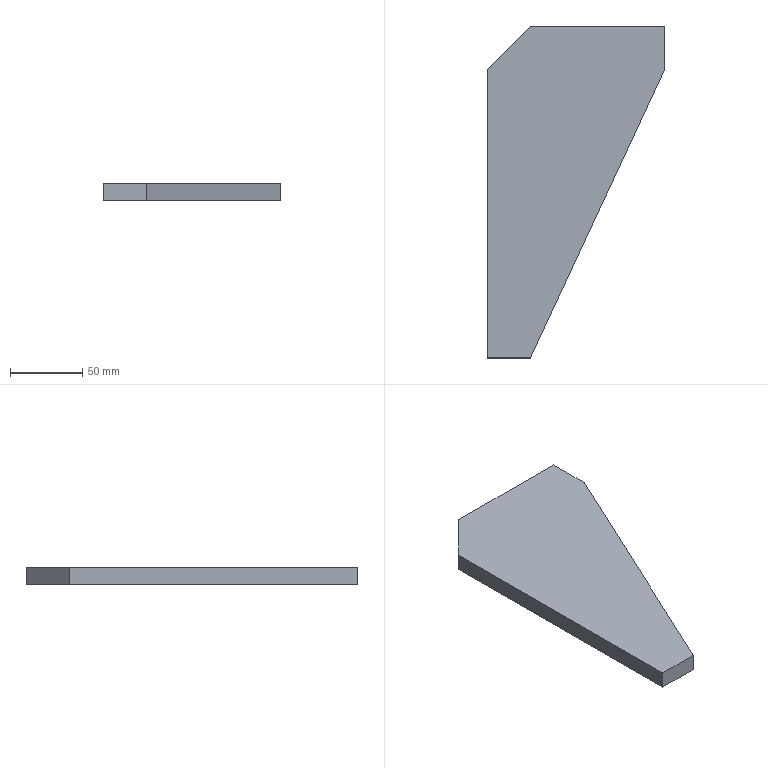Part | STEP file | Rib 6 | 1 solid | 8 faces | box 123 x 230 x 12 mm | volume 222480 mm3 | plane 8
STEP:
#1=CARTESIAN_POINT('',(0.,0.,0.));
#2=DIRECTION('',(0.,0.,1.));
#3=DIRECTION('',(1.,0.,0.));
#4=AXIS2_PLACEMENT_3D('',#1,#2,#3);
#5=CARTESIAN_POINT('',(152.,160.,0.));
#6=VERTEX_POINT('',#5);
#7=CARTESIAN_POINT('',(122.,130.,0.));
#8=VERTEX_POINT('',#7);
#9=CARTESIAN_POINT('',(152.,160.,0.));
#10=DIRECTION('',(-0.7071,-0.7071,0.));
#11=VECTOR('',#10,1.);
#12=LINE('',#9,#11);
#13=CARTESIAN_POINT('',(152.,160.,12.));
#14=DIRECTION('',(0.7071,-0.7071,0.));
#15=DIRECTION('',(0.7071,0.7071,0.));
#16=AXIS2_PLACEMENT_3D('',#13,#14,#15);
#17=PLANE('',#16);
#18=CARTESIAN_POINT('',(0.,-12.));
#19=DIRECTION('',(-1.,0.));
#20=VECTOR('',#19,1.);
#21=LINE('',#18,#20);
#22=(GEOMETRIC_REPRESENTATION_CONTEXT(2)PARAMETRIC_REPRESENTATION_CONTEXT()REPRESENTATION_CONTEXT('',''));
#23=DEFINITIONAL_REPRESENTATION('',(#21),#22);
#24=PCURVE('',#17,#23);
#25=CARTESIAN_POINT('',(122.,130.,0.));
#26=DIRECTION('',(0.,0.,1.));
#27=DIRECTION('',(1.,0.,0.));
#28=AXIS2_PLACEMENT_3D('',#25,#26,#27);
#29=PLANE('',#28);
#30=CARTESIAN_POINT('',(30.,30.));
#31=DIRECTION('',(-0.7071,-0.7071));
#32=VECTOR('',#31,1.);
#33=LINE('',#30,#32);
#34=(GEOMETRIC_REPRESENTATION_CONTEXT(2)PARAMETRIC_REPRESENTATION_CONTEXT()REPRESENTATION_CONTEXT('',''));
#35=DEFINITIONAL_REPRESENTATION('',(#33),#34);
#36=PCURVE('',#29,#35);
#37=SURFACE_CURVE('',#12,(#24,#36),.PCURVE_S1.);
#38=EDGE_CURVE('',#6,#8,#37,.T.);
#39=ORIENTED_EDGE('',*,*,#38,.T.);
#40=CARTESIAN_POINT('',(122.,130.,12.));
#41=VERTEX_POINT('',#40);
#42=CARTESIAN_POINT('',(122.,130.,12.));
#43=DIRECTION('',(0.,0.,-1.));
#44=VECTOR('',#43,1.);
#45=LINE('',#42,#44);
#46=CARTESIAN_POINT('',(-42.426,0.));
#47=DIRECTION('',(0.,-1.));
#48=VECTOR('',#47,1.);
#49=LINE('',#46,#48);
#50=(GEOMETRIC_REPRESENTATION_CONTEXT(2)PARAMETRIC_REPRESENTATION_CONTEXT()REPRESENTATION_CONTEXT('',''));
#51=DEFINITIONAL_REPRESENTATION('',(#49),#50);
#52=PCURVE('',#17,#51);
#53=CARTESIAN_POINT('',(122.,130.,12.));
#54=DIRECTION('',(1.,0.,0.));
#55=DIRECTION('',(0.,1.,0.));
#56=AXIS2_PLACEMENT_3D('',#53,#54,#55);
#57=PLANE('',#56);
#58=CARTESIAN_POINT('',(0.,0.));
#59=DIRECTION('',(0.,-1.));
#60=VECTOR('',#59,1.);
#61=LINE('',#58,#60);
#62=(GEOMETRIC_REPRESENTATION_CONTEXT(2)PARAMETRIC_REPRESENTATION_CONTEXT()REPRESENTATION_CONTEXT('',''));
#63=DEFINITIONAL_REPRESENTATION('',(#61),#62);
#64=PCURVE('',#57,#63);
#65=SURFACE_CURVE('',#45,(#52,#64),.PCURVE_S1.);
#66=EDGE_CURVE('',#41,#8,#65,.T.);
#67=ORIENTED_EDGE('',*,*,#66,.F.);
#68=CARTESIAN_POINT('',(152.,160.,12.));
#69=VERTEX_POINT('',#68);
#70=CARTESIAN_POINT('',(152.,160.,12.));
#71=DIRECTION('',(-0.7071,-0.7071,0.));
#72=VECTOR('',#71,1.);
#73=LINE('',#70,#72);
#74=CARTESIAN_POINT('',(0.,0.));
#75=DIRECTION('',(-1.,0.));
#76=VECTOR('',#75,1.);
#77=LINE('',#74,#76);
#78=(GEOMETRIC_REPRESENTATION_CONTEXT(2)PARAMETRIC_REPRESENTATION_CONTEXT()REPRESENTATION_CONTEXT('',''));
#79=DEFINITIONAL_REPRESENTATION('',(#77),#78);
#80=PCURVE('',#17,#79);
#81=CARTESIAN_POINT('',(122.,130.,12.));
#82=DIRECTION('',(0.,0.,1.));
#83=DIRECTION('',(1.,0.,0.));
#84=AXIS2_PLACEMENT_3D('',#81,#82,#83);
#85=PLANE('',#84);
#86=CARTESIAN_POINT('',(30.,30.));
#87=DIRECTION('',(-0.7071,-0.7071));
#88=VECTOR('',#87,1.);
#89=LINE('',#86,#88);
#90=(GEOMETRIC_REPRESENTATION_CONTEXT(2)PARAMETRIC_REPRESENTATION_CONTEXT()REPRESENTATION_CONTEXT('',''));
#91=DEFINITIONAL_REPRESENTATION('',(#89),#90);
#92=PCURVE('',#85,#91);
#93=SURFACE_CURVE('',#73,(#80,#92),.PCURVE_S1.);
#94=EDGE_CURVE('',#69,#41,#93,.T.);
#95=ORIENTED_EDGE('',*,*,#94,.F.);
#96=CARTESIAN_POINT('',(152.,160.,12.));
#97=DIRECTION('',(0.,0.,-1.));
#98=VECTOR('',#97,1.);
#99=LINE('',#96,#98);
#100=CARTESIAN_POINT('',(0.,0.));
#101=DIRECTION('',(0.,-1.));
#102=VECTOR('',#101,1.);
#103=LINE('',#100,#102);
#104=(GEOMETRIC_REPRESENTATION_CONTEXT(2)PARAMETRIC_REPRESENTATION_CONTEXT()REPRESENTATION_CONTEXT('',''));
#105=DEFINITIONAL_REPRESENTATION('',(#103),#104);
#106=PCURVE('',#17,#105);
#107=CARTESIAN_POINT('',(245.,160.,12.));
#108=DIRECTION('',(0.,-1.,0.));
#109=DIRECTION('',(0.,0.,-1.));
#110=AXIS2_PLACEMENT_3D('',#107,#108,#109);
#111=PLANE('',#110);
#112=CARTESIAN_POINT('',(0.,-93.));
#113=DIRECTION('',(1.,0.));
#114=VECTOR('',#113,1.);
#115=LINE('',#112,#114);
#116=(GEOMETRIC_REPRESENTATION_CONTEXT(2)PARAMETRIC_REPRESENTATION_CONTEXT()REPRESENTATION_CONTEXT('',''));
#117=DEFINITIONAL_REPRESENTATION('',(#115),#116);
#118=PCURVE('',#111,#117);
#119=SURFACE_CURVE('',#99,(#106,#118),.PCURVE_S1.);
#120=EDGE_CURVE('',#69,#6,#119,.T.);
#121=ORIENTED_EDGE('',*,*,#120,.T.);
#122=EDGE_LOOP('',(#39,#67,#95,#121));
#123=FACE_BOUND('',#122,.T.);
#124=ADVANCED_FACE('',(#123),#17,.F.);
#125=CARTESIAN_POINT('',(122.,-70.,0.));
#126=VERTEX_POINT('',#125);
#127=CARTESIAN_POINT('',(122.,130.,0.));
#128=DIRECTION('',(0.,-1.,0.));
#129=VECTOR('',#128,1.);
#130=LINE('',#127,#129);
#131=CARTESIAN_POINT('',(0.,-12.));
#132=DIRECTION('',(-1.,0.));
#133=VECTOR('',#132,1.);
#134=LINE('',#131,#133);
#135=(GEOMETRIC_REPRESENTATION_CONTEXT(2)PARAMETRIC_REPRESENTATION_CONTEXT()REPRESENTATION_CONTEXT('',''));
#136=DEFINITIONAL_REPRESENTATION('',(#134),#135);
#137=PCURVE('',#57,#136);
#138=CARTESIAN_POINT('',(0.,0.));
#139=DIRECTION('',(0.,-1.));
#140=VECTOR('',#139,1.);
#141=LINE('',#138,#140);
#142=(GEOMETRIC_REPRESENTATION_CONTEXT(2)PARAMETRIC_REPRESENTATION_CONTEXT()REPRESENTATION_CONTEXT('',''));
#143=DEFINITIONAL_REPRESENTATION('',(#141),#142);
#144=PCURVE('',#29,#143);
#145=SURFACE_CURVE('',#130,(#137,#144),.PCURVE_S1.);
#146=EDGE_CURVE('',#8,#126,#145,.T.);
#147=ORIENTED_EDGE('',*,*,#146,.T.);
#148=CARTESIAN_POINT('',(122.,-70.,12.));
#149=VERTEX_POINT('',#148);
#150=CARTESIAN_POINT('',(122.,-70.,12.));
#151=DIRECTION('',(0.,0.,-1.));
#152=VECTOR('',#151,1.);
#153=LINE('',#150,#152);
#154=CARTESIAN_POINT('',(-200.,0.));
#155=DIRECTION('',(0.,-1.));
#156=VECTOR('',#155,1.);
#157=LINE('',#154,#156);
#158=(GEOMETRIC_REPRESENTATION_CONTEXT(2)PARAMETRIC_REPRESENTATION_CONTEXT()REPRESENTATION_CONTEXT('',''));
#159=DEFINITIONAL_REPRESENTATION('',(#157),#158);
#160=PCURVE('',#57,#159);
#161=CARTESIAN_POINT('',(122.,-70.,12.));
#162=DIRECTION('',(0.,1.,0.));
#163=DIRECTION('',(0.,0.,1.));
#164=AXIS2_PLACEMENT_3D('',#161,#162,#163);
#165=PLANE('',#164);
#166=CARTESIAN_POINT('',(0.,0.));
#167=DIRECTION('',(-1.,0.));
#168=VECTOR('',#167,1.);
#169=LINE('',#166,#168);
#170=(GEOMETRIC_REPRESENTATION_CONTEXT(2)PARAMETRIC_REPRESENTATION_CONTEXT()REPRESENTATION_CONTEXT('',''));
#171=DEFINITIONAL_REPRESENTATION('',(#169),#170);
#172=PCURVE('',#165,#171);
#173=SURFACE_CURVE('',#153,(#160,#172),.PCURVE_S1.);
#174=EDGE_CURVE('',#149,#126,#173,.T.);
#175=ORIENTED_EDGE('',*,*,#174,.F.);
#176=CARTESIAN_POINT('',(122.,130.,12.));
#177=DIRECTION('',(0.,-1.,0.));
#178=VECTOR('',#177,1.);
#179=LINE('',#176,#178);
#180=CARTESIAN_POINT('',(0.,0.));
#181=DIRECTION('',(-1.,0.));
#182=VECTOR('',#181,1.);
#183=LINE('',#180,#182);
#184=(GEOMETRIC_REPRESENTATION_CONTEXT(2)PARAMETRIC_REPRESENTATION_CONTEXT()REPRESENTATION_CONTEXT('',''));
#185=DEFINITIONAL_REPRESENTATION('',(#183),#184);
#186=PCURVE('',#57,#185);
#187=CARTESIAN_POINT('',(0.,0.));
#188=DIRECTION('',(0.,-1.));
#189=VECTOR('',#188,1.);
#190=LINE('',#187,#189);
#191=(GEOMETRIC_REPRESENTATION_CONTEXT(2)PARAMETRIC_REPRESENTATION_CONTEXT()REPRESENTATION_CONTEXT('',''));
#192=DEFINITIONAL_REPRESENTATION('',(#190),#191);
#193=PCURVE('',#85,#192);
#194=SURFACE_CURVE('',#179,(#186,#193),.PCURVE_S1.);
#195=EDGE_CURVE('',#41,#149,#194,.T.);
#196=ORIENTED_EDGE('',*,*,#195,.F.);
#197=ORIENTED_EDGE('',*,*,#66,.T.);
#198=EDGE_LOOP('',(#147,#175,#196,#197));
#199=FACE_BOUND('',#198,.T.);
#200=ADVANCED_FACE('',(#199),#57,.F.);
#201=CARTESIAN_POINT('',(152.,-70.,0.));
#202=VERTEX_POINT('',#201);
#203=CARTESIAN_POINT('',(122.,-70.,0.));
#204=DIRECTION('',(1.,0.,0.));
#205=VECTOR('',#204,1.);
#206=LINE('',#203,#205);
#207=CARTESIAN_POINT('',(-12.,0.));
#208=DIRECTION('',(0.,1.));
#209=VECTOR('',#208,1.);
#210=LINE('',#207,#209);
#211=(GEOMETRIC_REPRESENTATION_CONTEXT(2)PARAMETRIC_REPRESENTATION_CONTEXT()REPRESENTATION_CONTEXT('',''));
#212=DEFINITIONAL_REPRESENTATION('',(#210),#211);
#213=PCURVE('',#165,#212);
#214=CARTESIAN_POINT('',(0.,-200.));
#215=DIRECTION('',(1.,0.));
#216=VECTOR('',#215,1.);
#217=LINE('',#214,#216);
#218=(GEOMETRIC_REPRESENTATION_CONTEXT(2)PARAMETRIC_REPRESENTATION_CONTEXT()REPRESENTATION_CONTEXT('',''));
#219=DEFINITIONAL_REPRESENTATION('',(#217),#218);
#220=PCURVE('',#29,#219);
#221=SURFACE_CURVE('',#206,(#213,#220),.PCURVE_S1.);
#222=EDGE_CURVE('',#126,#202,#221,.T.);
#223=ORIENTED_EDGE('',*,*,#222,.T.);
#224=CARTESIAN_POINT('',(152.,-70.,12.));
#225=VERTEX_POINT('',#224);
#226=CARTESIAN_POINT('',(152.,-70.,12.));
#227=DIRECTION('',(0.,0.,-1.));
#228=VECTOR('',#227,1.);
#229=LINE('',#226,#228);
#230=CARTESIAN_POINT('',(0.,30.));
#231=DIRECTION('',(-1.,0.));
#232=VECTOR('',#231,1.);
#233=LINE('',#230,#232);
#234=(GEOMETRIC_REPRESENTATION_CONTEXT(2)PARAMETRIC_REPRESENTATION_CONTEXT()REPRESENTATION_CONTEXT('',''));
#235=DEFINITIONAL_REPRESENTATION('',(#233),#234);
#236=PCURVE('',#165,#235);
#237=CARTESIAN_POINT('',(152.,-70.,12.));
#238=DIRECTION('',(-0.9068,0.4216,0.));
#239=DIRECTION('',(-0.4216,-0.9068,0.));
#240=AXIS2_PLACEMENT_3D('',#237,#238,#239);
#241=PLANE('',#240);
#242=CARTESIAN_POINT('',(0.,0.));
#243=DIRECTION('',(0.,-1.));
#244=VECTOR('',#243,1.);
#245=LINE('',#242,#244);
#246=(GEOMETRIC_REPRESENTATION_CONTEXT(2)PARAMETRIC_REPRESENTATION_CONTEXT()REPRESENTATION_CONTEXT('',''));
#247=DEFINITIONAL_REPRESENTATION('',(#245),#246);
#248=PCURVE('',#241,#247);
#249=SURFACE_CURVE('',#229,(#236,#248),.PCURVE_S1.);
#250=EDGE_CURVE('',#225,#202,#249,.T.);
#251=ORIENTED_EDGE('',*,*,#250,.F.);
#252=CARTESIAN_POINT('',(122.,-70.,12.));
#253=DIRECTION('',(1.,0.,0.));
#254=VECTOR('',#253,1.);
#255=LINE('',#252,#254);
#256=CARTESIAN_POINT('',(0.,0.));
#257=DIRECTION('',(0.,1.));
#258=VECTOR('',#257,1.);
#259=LINE('',#256,#258);
#260=(GEOMETRIC_REPRESENTATION_CONTEXT(2)PARAMETRIC_REPRESENTATION_CONTEXT()REPRESENTATION_CONTEXT('',''));
#261=DEFINITIONAL_REPRESENTATION('',(#259),#260);
#262=PCURVE('',#165,#261);
#263=CARTESIAN_POINT('',(0.,-200.));
#264=DIRECTION('',(1.,0.));
#265=VECTOR('',#264,1.);
#266=LINE('',#263,#265);
#267=(GEOMETRIC_REPRESENTATION_CONTEXT(2)PARAMETRIC_REPRESENTATION_CONTEXT()REPRESENTATION_CONTEXT('',''));
#268=DEFINITIONAL_REPRESENTATION('',(#266),#267);
#269=PCURVE('',#85,#268);
#270=SURFACE_CURVE('',#255,(#262,#269),.PCURVE_S1.);
#271=EDGE_CURVE('',#149,#225,#270,.T.);
#272=ORIENTED_EDGE('',*,*,#271,.F.);
#273=ORIENTED_EDGE('',*,*,#174,.T.);
#274=EDGE_LOOP('',(#223,#251,#272,#273));
#275=FACE_BOUND('',#274,.T.);
#276=ADVANCED_FACE('',(#275),#165,.F.);
#277=CARTESIAN_POINT('',(245.,130.,0.));
#278=VERTEX_POINT('',#277);
#279=CARTESIAN_POINT('',(152.,-70.,0.));
#280=DIRECTION('',(0.4216,0.9068,0.));
#281=VECTOR('',#280,1.);
#282=LINE('',#279,#281);
#283=CARTESIAN_POINT('',(0.,-12.));
#284=DIRECTION('',(-1.,0.));
#285=VECTOR('',#284,1.);
#286=LINE('',#283,#285);
#287=(GEOMETRIC_REPRESENTATION_CONTEXT(2)PARAMETRIC_REPRESENTATION_CONTEXT()REPRESENTATION_CONTEXT('',''));
#288=DEFINITIONAL_REPRESENTATION('',(#286),#287);
#289=PCURVE('',#241,#288);
#290=CARTESIAN_POINT('',(30.,-200.));
#291=DIRECTION('',(0.4216,0.9068));
#292=VECTOR('',#291,1.);
#293=LINE('',#290,#292);
#294=(GEOMETRIC_REPRESENTATION_CONTEXT(2)PARAMETRIC_REPRESENTATION_CONTEXT()REPRESENTATION_CONTEXT('',''));
#295=DEFINITIONAL_REPRESENTATION('',(#293),#294);
#296=PCURVE('',#29,#295);
#297=SURFACE_CURVE('',#282,(#289,#296),.PCURVE_S1.);
#298=EDGE_CURVE('',#202,#278,#297,.T.);
#299=ORIENTED_EDGE('',*,*,#298,.T.);
#300=CARTESIAN_POINT('',(245.,130.,12.));
#301=VERTEX_POINT('',#300);
#302=CARTESIAN_POINT('',(245.,130.,12.));
#303=DIRECTION('',(0.,0.,-1.));
#304=VECTOR('',#303,1.);
#305=LINE('',#302,#304);
#306=CARTESIAN_POINT('',(-220.565,0.));
#307=DIRECTION('',(0.,-1.));
#308=VECTOR('',#307,1.);
#309=LINE('',#306,#308);
#310=(GEOMETRIC_REPRESENTATION_CONTEXT(2)PARAMETRIC_REPRESENTATION_CONTEXT()REPRESENTATION_CONTEXT('',''));
#311=DEFINITIONAL_REPRESENTATION('',(#309),#310);
#312=PCURVE('',#241,#311);
#313=CARTESIAN_POINT('',(245.,130.,12.));
#314=DIRECTION('',(-1.,0.,0.));
#315=DIRECTION('',(0.,0.,1.));
#316=AXIS2_PLACEMENT_3D('',#313,#314,#315);
#317=PLANE('',#316);
#318=CARTESIAN_POINT('',(0.,0.));
#319=DIRECTION('',(-1.,0.));
#320=VECTOR('',#319,1.);
#321=LINE('',#318,#320);
#322=(GEOMETRIC_REPRESENTATION_CONTEXT(2)PARAMETRIC_REPRESENTATION_CONTEXT()REPRESENTATION_CONTEXT('',''));
#323=DEFINITIONAL_REPRESENTATION('',(#321),#322);
#324=PCURVE('',#317,#323);
#325=SURFACE_CURVE('',#305,(#312,#324),.PCURVE_S1.);
#326=EDGE_CURVE('',#301,#278,#325,.T.);
#327=ORIENTED_EDGE('',*,*,#326,.F.);
#328=CARTESIAN_POINT('',(152.,-70.,12.));
#329=DIRECTION('',(0.4216,0.9068,0.));
#330=VECTOR('',#329,1.);
#331=LINE('',#328,#330);
#332=CARTESIAN_POINT('',(0.,0.));
#333=DIRECTION('',(-1.,0.));
#334=VECTOR('',#333,1.);
#335=LINE('',#332,#334);
#336=(GEOMETRIC_REPRESENTATION_CONTEXT(2)PARAMETRIC_REPRESENTATION_CONTEXT()REPRESENTATION_CONTEXT('',''));
#337=DEFINITIONAL_REPRESENTATION('',(#335),#336);
#338=PCURVE('',#241,#337);
#339=CARTESIAN_POINT('',(30.,-200.));
#340=DIRECTION('',(0.4216,0.9068));
#341=VECTOR('',#340,1.);
#342=LINE('',#339,#341);
#343=(GEOMETRIC_REPRESENTATION_CONTEXT(2)PARAMETRIC_REPRESENTATION_CONTEXT()REPRESENTATION_CONTEXT('',''));
#344=DEFINITIONAL_REPRESENTATION('',(#342),#343);
#345=PCURVE('',#85,#344);
#346=SURFACE_CURVE('',#331,(#338,#345),.PCURVE_S1.);
#347=EDGE_CURVE('',#225,#301,#346,.T.);
#348=ORIENTED_EDGE('',*,*,#347,.F.);
#349=ORIENTED_EDGE('',*,*,#250,.T.);
#350=EDGE_LOOP('',(#299,#327,#348,#349));
#351=FACE_BOUND('',#350,.T.);
#352=ADVANCED_FACE('',(#351),#241,.F.);
#353=CARTESIAN_POINT('',(245.,160.,0.));
#354=VERTEX_POINT('',#353);
#355=CARTESIAN_POINT('',(245.,130.,0.));
#356=DIRECTION('',(0.,1.,0.));
#357=VECTOR('',#356,1.);
#358=LINE('',#355,#357);
#359=CARTESIAN_POINT('',(-12.,0.));
#360=DIRECTION('',(0.,1.));
#361=VECTOR('',#360,1.);
#362=LINE('',#359,#361);
#363=(GEOMETRIC_REPRESENTATION_CONTEXT(2)PARAMETRIC_REPRESENTATION_CONTEXT()REPRESENTATION_CONTEXT('',''));
#364=DEFINITIONAL_REPRESENTATION('',(#362),#363);
#365=PCURVE('',#317,#364);
#366=CARTESIAN_POINT('',(123.,0.));
#367=DIRECTION('',(0.,1.));
#368=VECTOR('',#367,1.);
#369=LINE('',#366,#368);
#370=(GEOMETRIC_REPRESENTATION_CONTEXT(2)PARAMETRIC_REPRESENTATION_CONTEXT()REPRESENTATION_CONTEXT('',''));
#371=DEFINITIONAL_REPRESENTATION('',(#369),#370);
#372=PCURVE('',#29,#371);
#373=SURFACE_CURVE('',#358,(#365,#372),.PCURVE_S1.);
#374=EDGE_CURVE('',#278,#354,#373,.T.);
#375=ORIENTED_EDGE('',*,*,#374,.T.);
#376=CARTESIAN_POINT('',(245.,160.,12.));
#377=VERTEX_POINT('',#376);
#378=CARTESIAN_POINT('',(245.,160.,12.));
#379=DIRECTION('',(0.,0.,-1.));
#380=VECTOR('',#379,1.);
#381=LINE('',#378,#380);
#382=CARTESIAN_POINT('',(0.,30.));
#383=DIRECTION('',(-1.,0.));
#384=VECTOR('',#383,1.);
#385=LINE('',#382,#384);
#386=(GEOMETRIC_REPRESENTATION_CONTEXT(2)PARAMETRIC_REPRESENTATION_CONTEXT()REPRESENTATION_CONTEXT('',''));
#387=DEFINITIONAL_REPRESENTATION('',(#385),#386);
#388=PCURVE('',#317,#387);
#389=CARTESIAN_POINT('',(0.,0.));
#390=DIRECTION('',(1.,0.));
#391=VECTOR('',#390,1.);
#392=LINE('',#389,#391);
#393=(GEOMETRIC_REPRESENTATION_CONTEXT(2)PARAMETRIC_REPRESENTATION_CONTEXT()REPRESENTATION_CONTEXT('',''));
#394=DEFINITIONAL_REPRESENTATION('',(#392),#393);
#395=PCURVE('',#111,#394);
#396=SURFACE_CURVE('',#381,(#388,#395),.PCURVE_S1.);
#397=EDGE_CURVE('',#377,#354,#396,.T.);
#398=ORIENTED_EDGE('',*,*,#397,.F.);
#399=CARTESIAN_POINT('',(245.,130.,12.));
#400=DIRECTION('',(0.,1.,0.));
#401=VECTOR('',#400,1.);
#402=LINE('',#399,#401);
#403=CARTESIAN_POINT('',(0.,0.));
#404=DIRECTION('',(0.,1.));
#405=VECTOR('',#404,1.);
#406=LINE('',#403,#405);
#407=(GEOMETRIC_REPRESENTATION_CONTEXT(2)PARAMETRIC_REPRESENTATION_CONTEXT()REPRESENTATION_CONTEXT('',''));
#408=DEFINITIONAL_REPRESENTATION('',(#406),#407);
#409=PCURVE('',#317,#408);
#410=CARTESIAN_POINT('',(123.,0.));
#411=DIRECTION('',(0.,1.));
#412=VECTOR('',#411,1.);
#413=LINE('',#410,#412);
#414=(GEOMETRIC_REPRESENTATION_CONTEXT(2)PARAMETRIC_REPRESENTATION_CONTEXT()REPRESENTATION_CONTEXT('',''));
#415=DEFINITIONAL_REPRESENTATION('',(#413),#414);
#416=PCURVE('',#85,#415);
#417=SURFACE_CURVE('',#402,(#409,#416),.PCURVE_S1.);
#418=EDGE_CURVE('',#301,#377,#417,.T.);
#419=ORIENTED_EDGE('',*,*,#418,.F.);
#420=ORIENTED_EDGE('',*,*,#326,.T.);
#421=EDGE_LOOP('',(#375,#398,#419,#420));
#422=FACE_BOUND('',#421,.T.);
#423=ADVANCED_FACE('',(#422),#317,.F.);
#424=CARTESIAN_POINT('',(245.,160.,0.));
#425=DIRECTION('',(-1.,0.,0.));
#426=VECTOR('',#425,1.);
#427=LINE('',#424,#426);
#428=CARTESIAN_POINT('',(12.,0.));
#429=DIRECTION('',(0.,-1.));
#430=VECTOR('',#429,1.);
#431=LINE('',#428,#430);
#432=(GEOMETRIC_REPRESENTATION_CONTEXT(2)PARAMETRIC_REPRESENTATION_CONTEXT()REPRESENTATION_CONTEXT('',''));
#433=DEFINITIONAL_REPRESENTATION('',(#431),#432);
#434=PCURVE('',#111,#433);
#435=CARTESIAN_POINT('',(123.,30.));
#436=DIRECTION('',(-1.,0.));
#437=VECTOR('',#436,1.);
#438=LINE('',#435,#437);
#439=(GEOMETRIC_REPRESENTATION_CONTEXT(2)PARAMETRIC_REPRESENTATION_CONTEXT()REPRESENTATION_CONTEXT('',''));
#440=DEFINITIONAL_REPRESENTATION('',(#438),#439);
#441=PCURVE('',#29,#440);
#442=SURFACE_CURVE('',#427,(#434,#441),.PCURVE_S1.);
#443=EDGE_CURVE('',#354,#6,#442,.T.);
#444=ORIENTED_EDGE('',*,*,#443,.T.);
#445=ORIENTED_EDGE('',*,*,#120,.F.);
#446=CARTESIAN_POINT('',(245.,160.,12.));
#447=DIRECTION('',(-1.,0.,0.));
#448=VECTOR('',#447,1.);
#449=LINE('',#446,#448);
#450=CARTESIAN_POINT('',(0.,0.));
#451=DIRECTION('',(0.,-1.));
#452=VECTOR('',#451,1.);
#453=LINE('',#450,#452);
#454=(GEOMETRIC_REPRESENTATION_CONTEXT(2)PARAMETRIC_REPRESENTATION_CONTEXT()REPRESENTATION_CONTEXT('',''));
#455=DEFINITIONAL_REPRESENTATION('',(#453),#454);
#456=PCURVE('',#111,#455);
#457=CARTESIAN_POINT('',(123.,30.));
#458=DIRECTION('',(-1.,0.));
#459=VECTOR('',#458,1.);
#460=LINE('',#457,#459);
#461=(GEOMETRIC_REPRESENTATION_CONTEXT(2)PARAMETRIC_REPRESENTATION_CONTEXT()REPRESENTATION_CONTEXT('',''));
#462=DEFINITIONAL_REPRESENTATION('',(#460),#461);
#463=PCURVE('',#85,#462);
#464=SURFACE_CURVE('',#449,(#456,#463),.PCURVE_S1.);
#465=EDGE_CURVE('',#377,#69,#464,.T.);
#466=ORIENTED_EDGE('',*,*,#465,.F.);
#467=ORIENTED_EDGE('',*,*,#397,.T.);
#468=EDGE_LOOP('',(#444,#445,#466,#467));
#469=FACE_BOUND('',#468,.T.);
#470=ADVANCED_FACE('',(#469),#111,.F.);
#471=ORIENTED_EDGE('',*,*,#94,.T.);
#472=ORIENTED_EDGE('',*,*,#195,.T.);
#473=ORIENTED_EDGE('',*,*,#271,.T.);
#474=ORIENTED_EDGE('',*,*,#347,.T.);
#475=ORIENTED_EDGE('',*,*,#418,.T.);
#476=ORIENTED_EDGE('',*,*,#465,.T.);
#477=EDGE_LOOP('',(#471,#472,#473,#474,#475,#476));
#478=FACE_BOUND('',#477,.T.);
#479=ADVANCED_FACE('',(#478),#85,.T.);
#480=ORIENTED_EDGE('',*,*,#38,.F.);
#481=ORIENTED_EDGE('',*,*,#443,.F.);
#482=ORIENTED_EDGE('',*,*,#374,.F.);
#483=ORIENTED_EDGE('',*,*,#298,.F.);
#484=ORIENTED_EDGE('',*,*,#222,.F.);
#485=ORIENTED_EDGE('',*,*,#146,.F.);
#486=EDGE_LOOP('',(#480,#481,#482,#483,#484,#485));
#487=FACE_BOUND('',#486,.T.);
#488=ADVANCED_FACE('',(#487),#29,.F.);
#489=CLOSED_SHELL('',(#124,#200,#276,#352,#423,#470,#479,#488));
#490=MANIFOLD_SOLID_BREP('',#489);
#491=(LENGTH_UNIT()NAMED_UNIT(*)SI_UNIT(.MILLI.,.METRE.));
#492=UNCERTAINTY_MEASURE_WITH_UNIT(LENGTH_MEASURE(0.0000001),#491,'','');
#493=(NAMED_UNIT(*)PLANE_ANGLE_UNIT()SI_UNIT($,.RADIAN.));
#494=(NAMED_UNIT(*)SI_UNIT($,.STERADIAN.)SOLID_ANGLE_UNIT());
#495=(GEOMETRIC_REPRESENTATION_CONTEXT(3)GLOBAL_UNCERTAINTY_ASSIGNED_CONTEXT((#492))GLOBAL_UNIT_ASSIGNED_CONTEXT((#491,#493,#494))REPRESENTATION_CONTEXT('',''));
#496=ADVANCED_BREP_SHAPE_REPRESENTATION('',(#4,#490),#495);